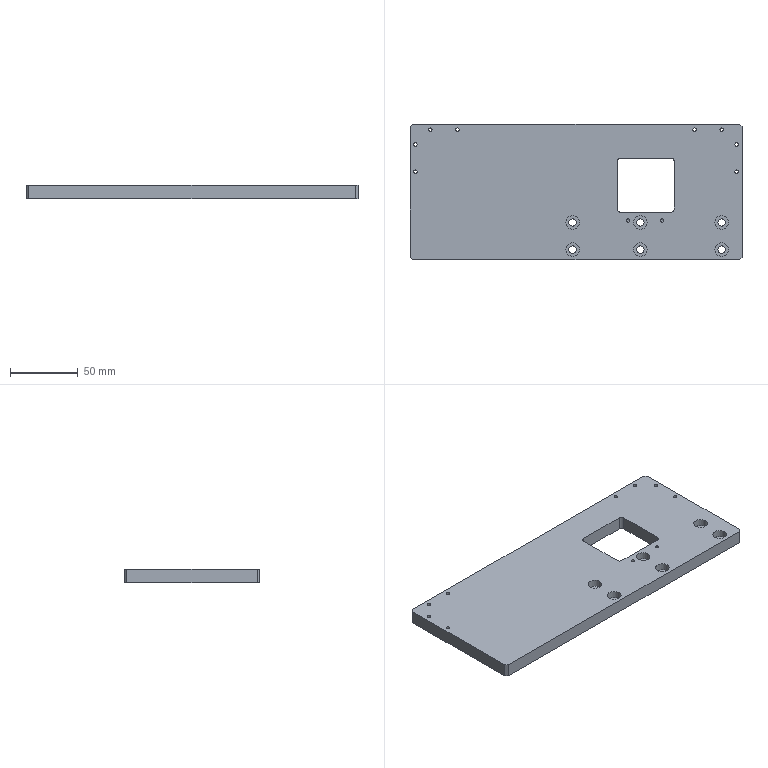CAM job | NX | 3-axis milling, drilling | part box 245 x 100 x 10 mm | stock box 250 x 105 x 12 mm
Tools:
number,name,description,diameter,corner_radius,flute_length,length,flutes
6,D6,平底铣刀-粗,6.0,0.0,25.0,75.0,2
9,D10,平底铣刀-粗,10.0,0.0,35.0,75.0,2
11,D4-J,平底铣刀-精,4.0,0.0,50.0,75.0,2
7,D6-J,平底铣刀-精,6.0,0.0,25.0,75.0,2
10,D10-J,平底铣刀-精,10.0,0.0,35.0,75.0,2
1,D80R0.8飞刀,圆鼻刀-粗,80.0,0.8,50.0,75.0,2
2,D6倒角刀,倒角刀,6.0,0.0,3.0,25.0,2
20,M3X0.5,丝锥,2.5,0.0,35.0,50.0,2
12,ZT2.5,钻头,2.5,0.0,35.0,50.0,2
17,ZT5.5,钻头,5.5,0.0,35.0,50.0,2
Operations:
program,operation,operation_type,tool,method,geometry_group,spindle_rpm,surface_speed,feed_per_tooth,feed_cut,feed_plunge,cut_length_mm,path_length_mm,cut_time_min,machine_time_min
B,面铣自动飞面开粗_COPY,FaceMilling,D80R0.8飞刀,分层开粗-切深K-步距G,W-B,4500.0,890.615,0.3333,3000.0,100.0,4322.556,5448.459,1.441,1.553
B,面铣自动飞面精光_COPY,FaceMilling,D80R0.8飞刀,侧刃精光-切深K-步距G,W-B,4500.0,890.615,0.1111,1000.0,100.0,1093.0,1129.0,1.093,1.097
B,钻倒角_2,Operation,D6倒角刀,METHOD,W-B,8000.0,150.796,0.0625,1000.0,0.0,38.0,424.607,0.038,0.0767
B,铣倒角_2,PlanarMilling,D6倒角刀,METHOD,W-B,8000.0,150.796,0.075,1200.0,100.0,106.768,528.892,0.089,0.1312
B,C0.3封闭铣廓倒角6X45L_COPY,PlanarMilling,D6倒角刀,爬面_倒角-切深0-步距G,W-B,7000.0,131.0,0.1071,1500.0,100.0,871.496,1117.122,0.581,0.6056
A,顶面,FaceMilling,D80R0.8飞刀,侧刃精光-切深K-步距G,W-A,4000.0,1005.31,0.125,1000.0,100.0,1079.0,1115.0,1.079,1.083
A,外形粗_2,VolumeBased25DMillingOperation,D10,METHOD,W-A,8000.0,251.327,0.3125,5000.0,80.0,10761.875,10810.475,2.152,2.157
A,框开粗_1,VolumeBased25DMillingOperation,D10,METHOD,W-A,6000.0,188.0,0.25,4000.0,80.0,2711.921,2760.22,0.678,0.6828
A,打点-深0.8,Operation,D6倒角刀,NONE,W-A,8000.0,150.796,0.0312,500.0,90.0,28.8,559.792,0.0576,0.1107
A,通孔-M3螺纹底孔,Operation,ZT2.5,NONE,W-A,3000.0,23.562,0.05,300.0,90.0,134.009,601.297,0.4467,0.4934
A,盲锥孔-M3螺纹底孔,Operation,ZT2.5,NONE,W-A,3000.0,23.562,0.0167,100.0,90.0,20.0,106.02,0.2,0.2086
A,沉头孔-钻孔0段,Operation,ZT5.5,NONE,W-A,1200.0,20.735,0.0625,150.0,90.0,87.914,390.922,0.5861,0.6164
A,铣孔开粗D6_1,CylinderMilling,D6,NONE,W-A,8000.0,150.796,0.075,1200.0,100.0,953.398,1392.798,0.7945,0.8384
A,铣孔精光D6_1,CylinderMilling,D6-J,精光步距切深关,W-A,8000.0,150.796,0.0312,500.0,100.0,200.391,642.791,0.4008,0.445
A,清角D4,ZLevelMilling,D4-J,METHOD,W-A,6000.0,75.0,0.25,2500.0,80.0,1489.114,1674.173,0.5961,0.6146
A,框精_1,VolumeBased25DMillingOperation,D6-J,METHOD,W-A,6000.0,113.0,0.0833,1000.0,100.0,144.842,203.442,0.1448,0.1507
A,仅选体,SurfaceContour,D6倒角刀,METHOD,W-A,8000.0,150.796,0.1875,3000.0,100.0,863.413,999.77,0.2878,0.3014
A,钻倒角_1,Operation,D6倒角刀,METHOD,W-A,8000.0,150.796,0.0312,500.0,0.0,47.5,508.301,0.095,0.1411
A,铣倒角_1,PlanarMilling,D6倒角刀,NONE,W-A,8000.0,150.796,0.05,800.0,100.0,241.506,641.551,0.3019,0.3419
A,通孔-攻牙M3,Operation,M3X0.5,METHOD,W-A,800.0,6.283,0.0003,0.5,90.0,112.0,557.28,224.0,224.044
A,盲锥孔-攻牙M3,Operation,M3X0.5,METHOD,W-A,1000.0,7.854,0.0003,0.5,90.0,15.0,96.02,30.0,30.008
A,外形半精_2,VolumeBased25DMillingOperation,D10-J,METHOD,W-A,8000.0,251.327,0.0625,1000.0,100.0,721.688,780.888,0.7217,0.7276